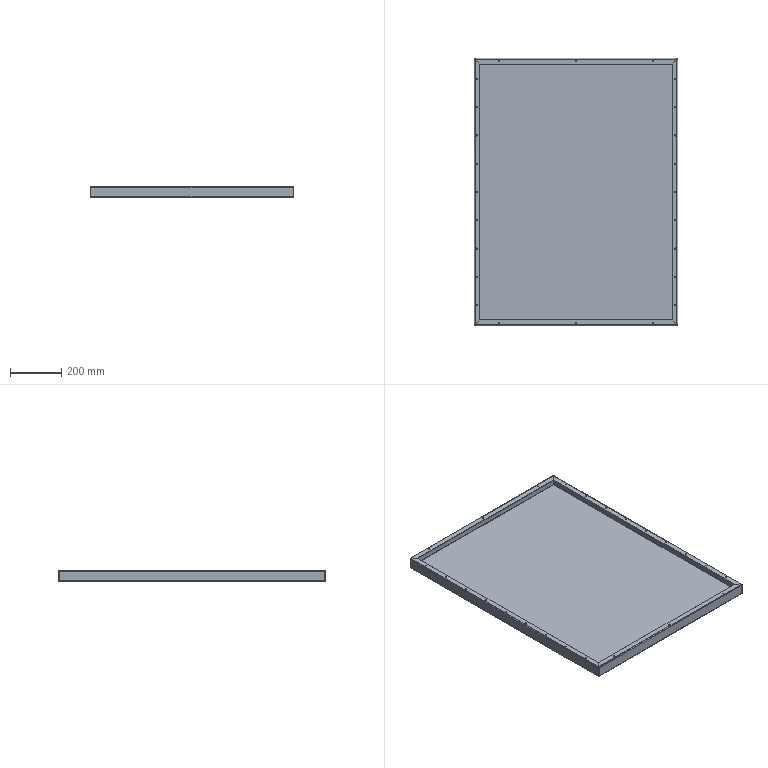Part | SolidWorks | 1 solid | 118 faces | box 794 x 1043 x 45 mm | volume 2619556 mm3 | cylinder 64 | plane 38 | spline 16 | commonest cylinder face diameters 5 x48 1.473 x8 6.473 x8